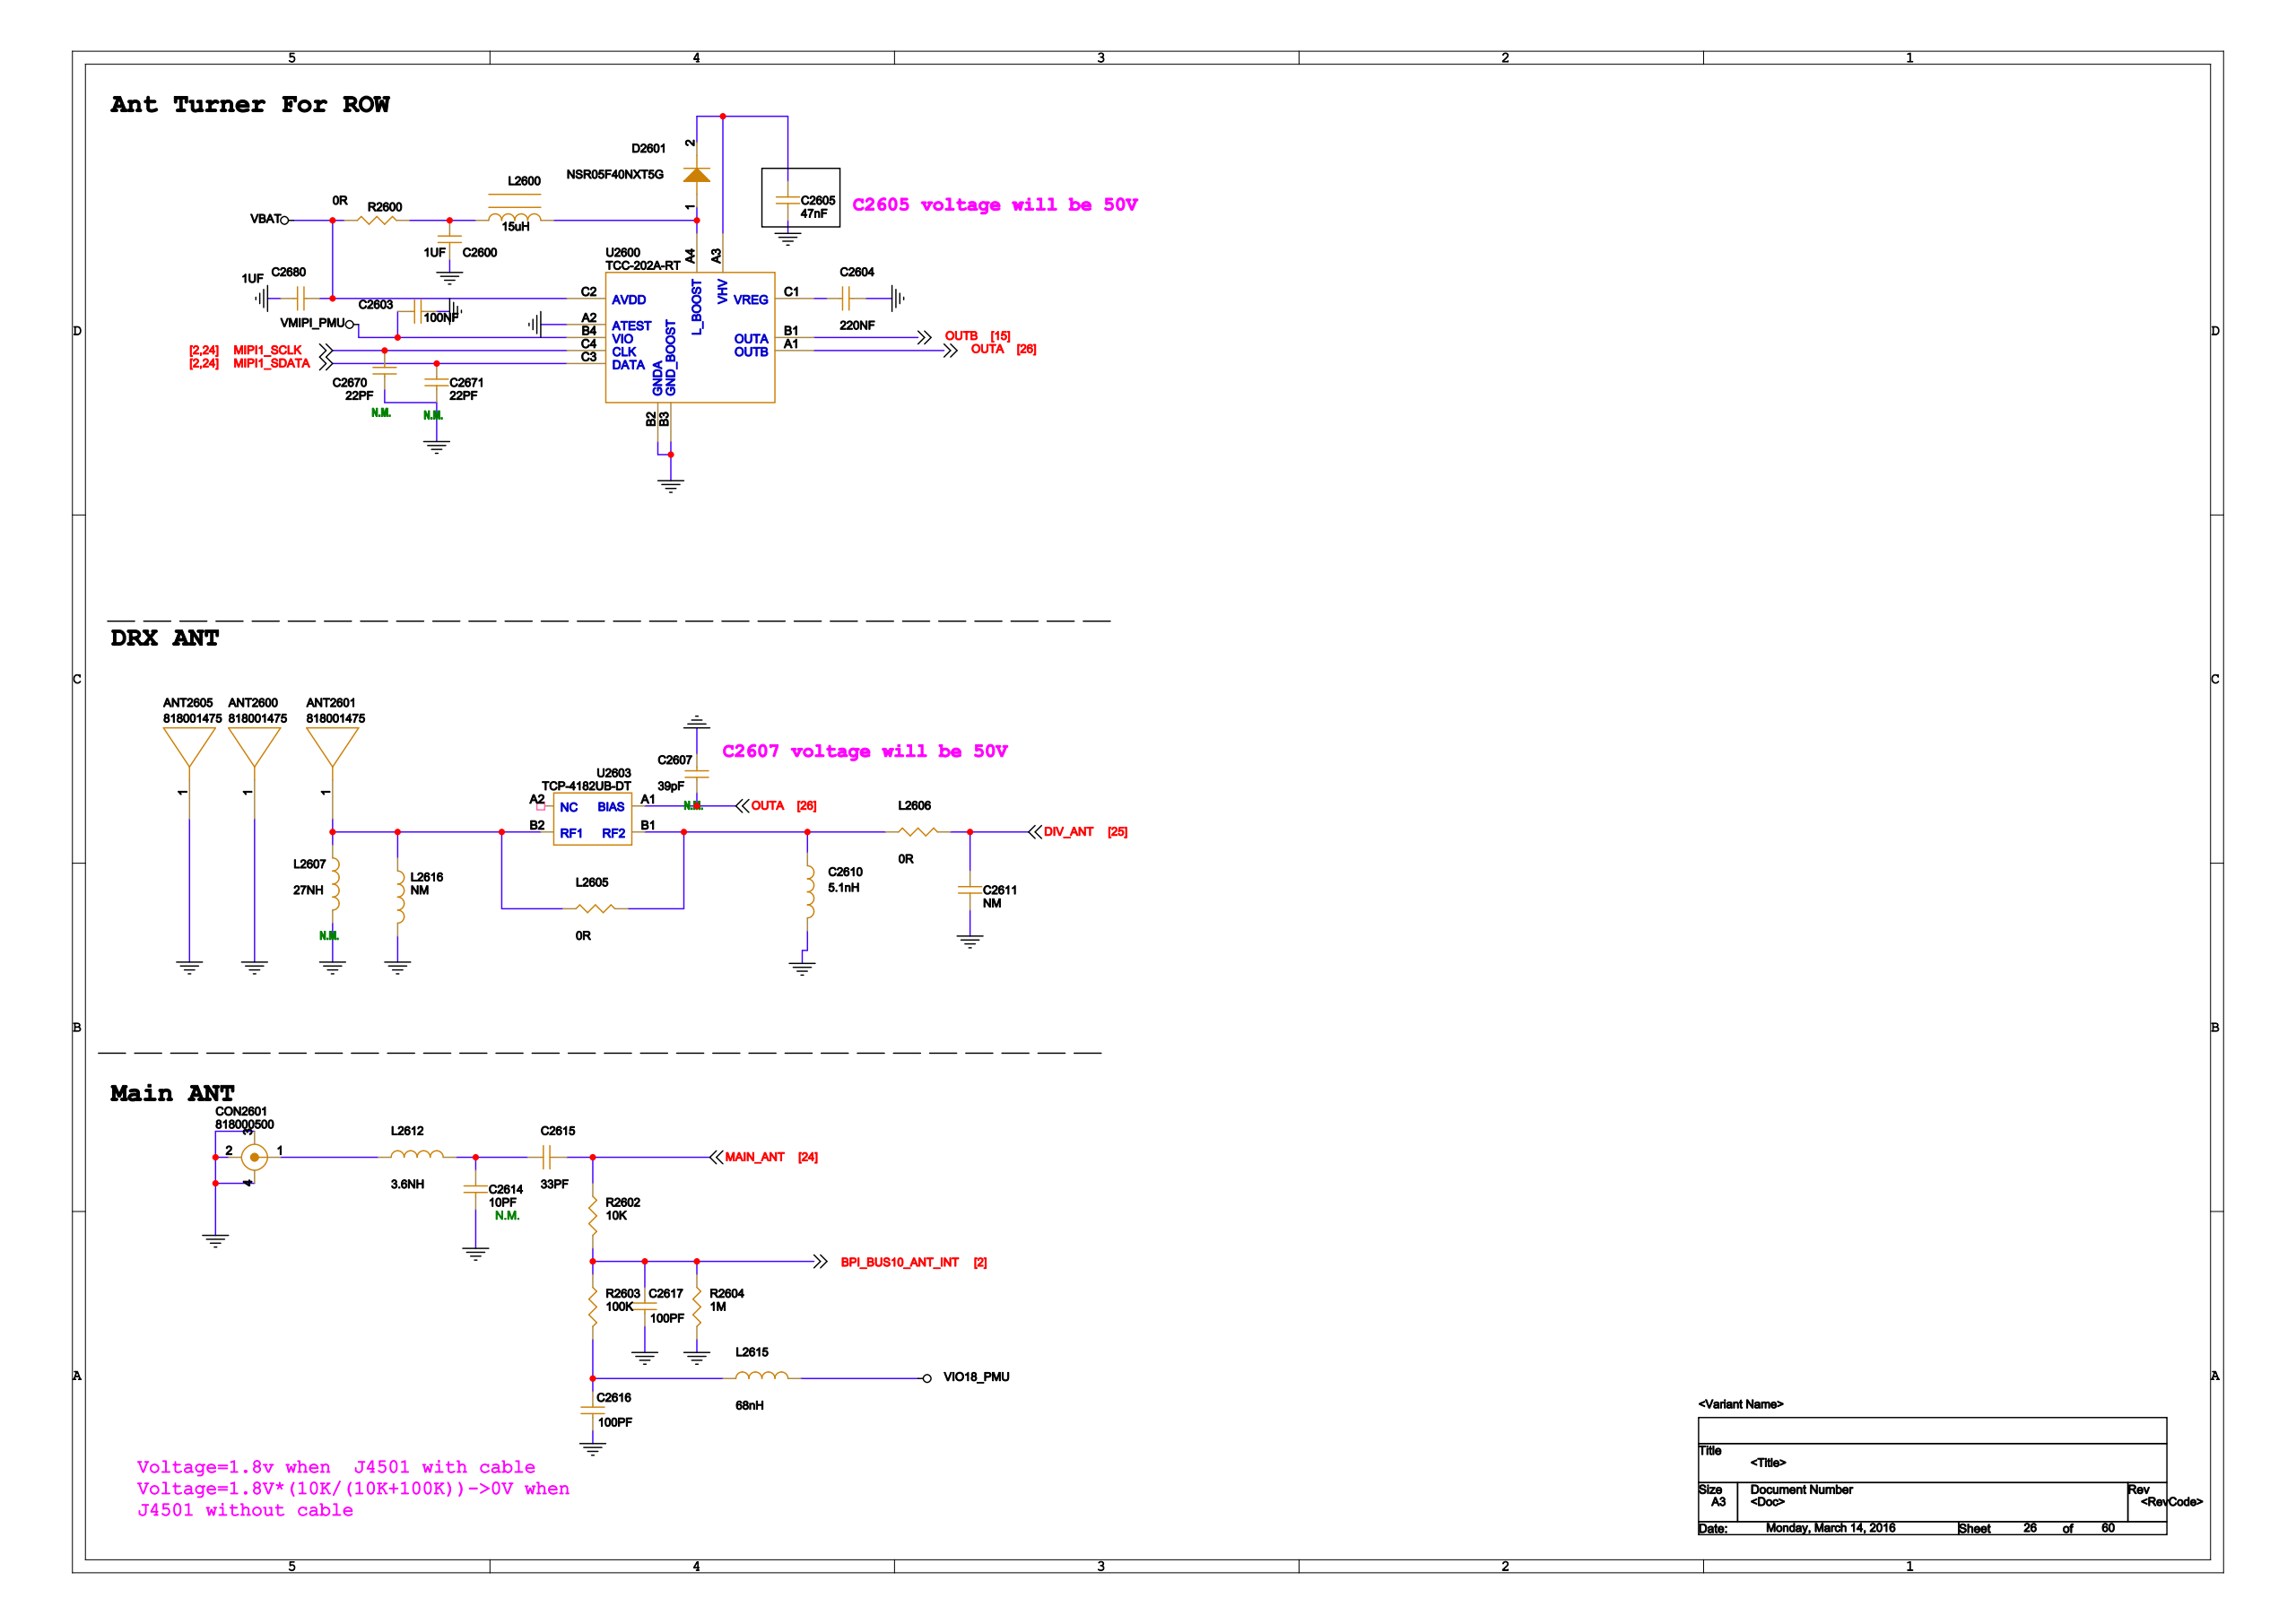Circuit board | Cadence Allegro | 1088 parts | 793 nets | one sheet of the schematic
Parts on this sheet (reference | value | footprint):
ANT2600 | 818001475 | PIN_ANT_818001475
ANT2601 | 818001475 | PIN_ANT_818001475
ANT2605 | 818001475 | PIN_ANT_818001475
C2600 | 1UF | C0201
C2603 | 100NF | C0201
C2604 | 220NF | C0201
C2605 | 47nF | C0402
C2607
C2610 | 5.1nH | L0201
C2611 | NM | 0201_NM
C2614
C2615 | 33PF | C0201
C2616 | 100PF | C0201
C2617 | 100PF | C0201
C2670
C2671
C2680 | 1UF | C0201
CON2601 | 818000500 | RF_818000500
D2601 | NSR05F40NXT5G | DSN2
L2600 | 15uH | L2016_VLS201610CX
L2605 | 0R | R0201
L2606 | 0R | R0201
L2607
L2612 | 3.6NH | L0201
L2615 | 68nH | L0201
L2616 | NM | 0201_NM
R2600 | 0R | R0201
R2602 | 10K | R0201
R2603 | 100K | R0201
R2604 | 1M | R0201
U2600 | TCC-202A-RT | WLCSP12_1P28X1P684X0P75_0P4
U2603 | TCP-4182UB-DT | WLCSP4_0P609X1P009X0P445
Nets of these parts (net: part-pin ...):
N35475291: C2605-1 D2601-2 U2600-A3
GND: ANT2600-1 ANT2605-1 C2600-2 C2603-1 C2604-2 C2605-2 C2607-2 C2610-2 C2611-2 C2614-2 C2616-2 C2617-2 C2670-1 C2671-2 C2680-2 CON2601-2 CON2601-3 CON2601-4 L2607-1 L2616-2 R2604-2 U2600-A2 U2600-B2 U2600-B3
N35475297: D2601-1 L2600-1 U2600-A4
VBAT: C2680-1 R2600-2 U2600-C2
MIPI1_SCLK: C2670-2 U2600-C4
MIPI1_SDATA: C2671-1 U2600-C3
OUTB: U2600-B1
OUTA: C2607-1 U2600-A1 U2603-A1
VMIPI_PMU: C2603-2 U2600-B4
N35475444: C2604-1 U2600-C1
N35412326: ANT2601-1 L2605-1 L2607-2 L2616-1 U2603-B2
N35412314: C2610-1 L2605-2 L2606-1 U2603-B1
MAIN_ANT: C2615-2 R2602-1
DIV_ANT: C2611-1 L2606-2
N33290355: CON2601-1 L2612-1
BPI_BUS10_ANT_INT: C2617-1 R2602-2 R2603-1 R2604-1
VIO18_PMU: L2615-2
N35475295: C2600-1 L2600-2 R2600-1
N33290357: C2614-1 C2615-1 L2612-2
N33289851: C2616-1 L2615-1 R2603-2